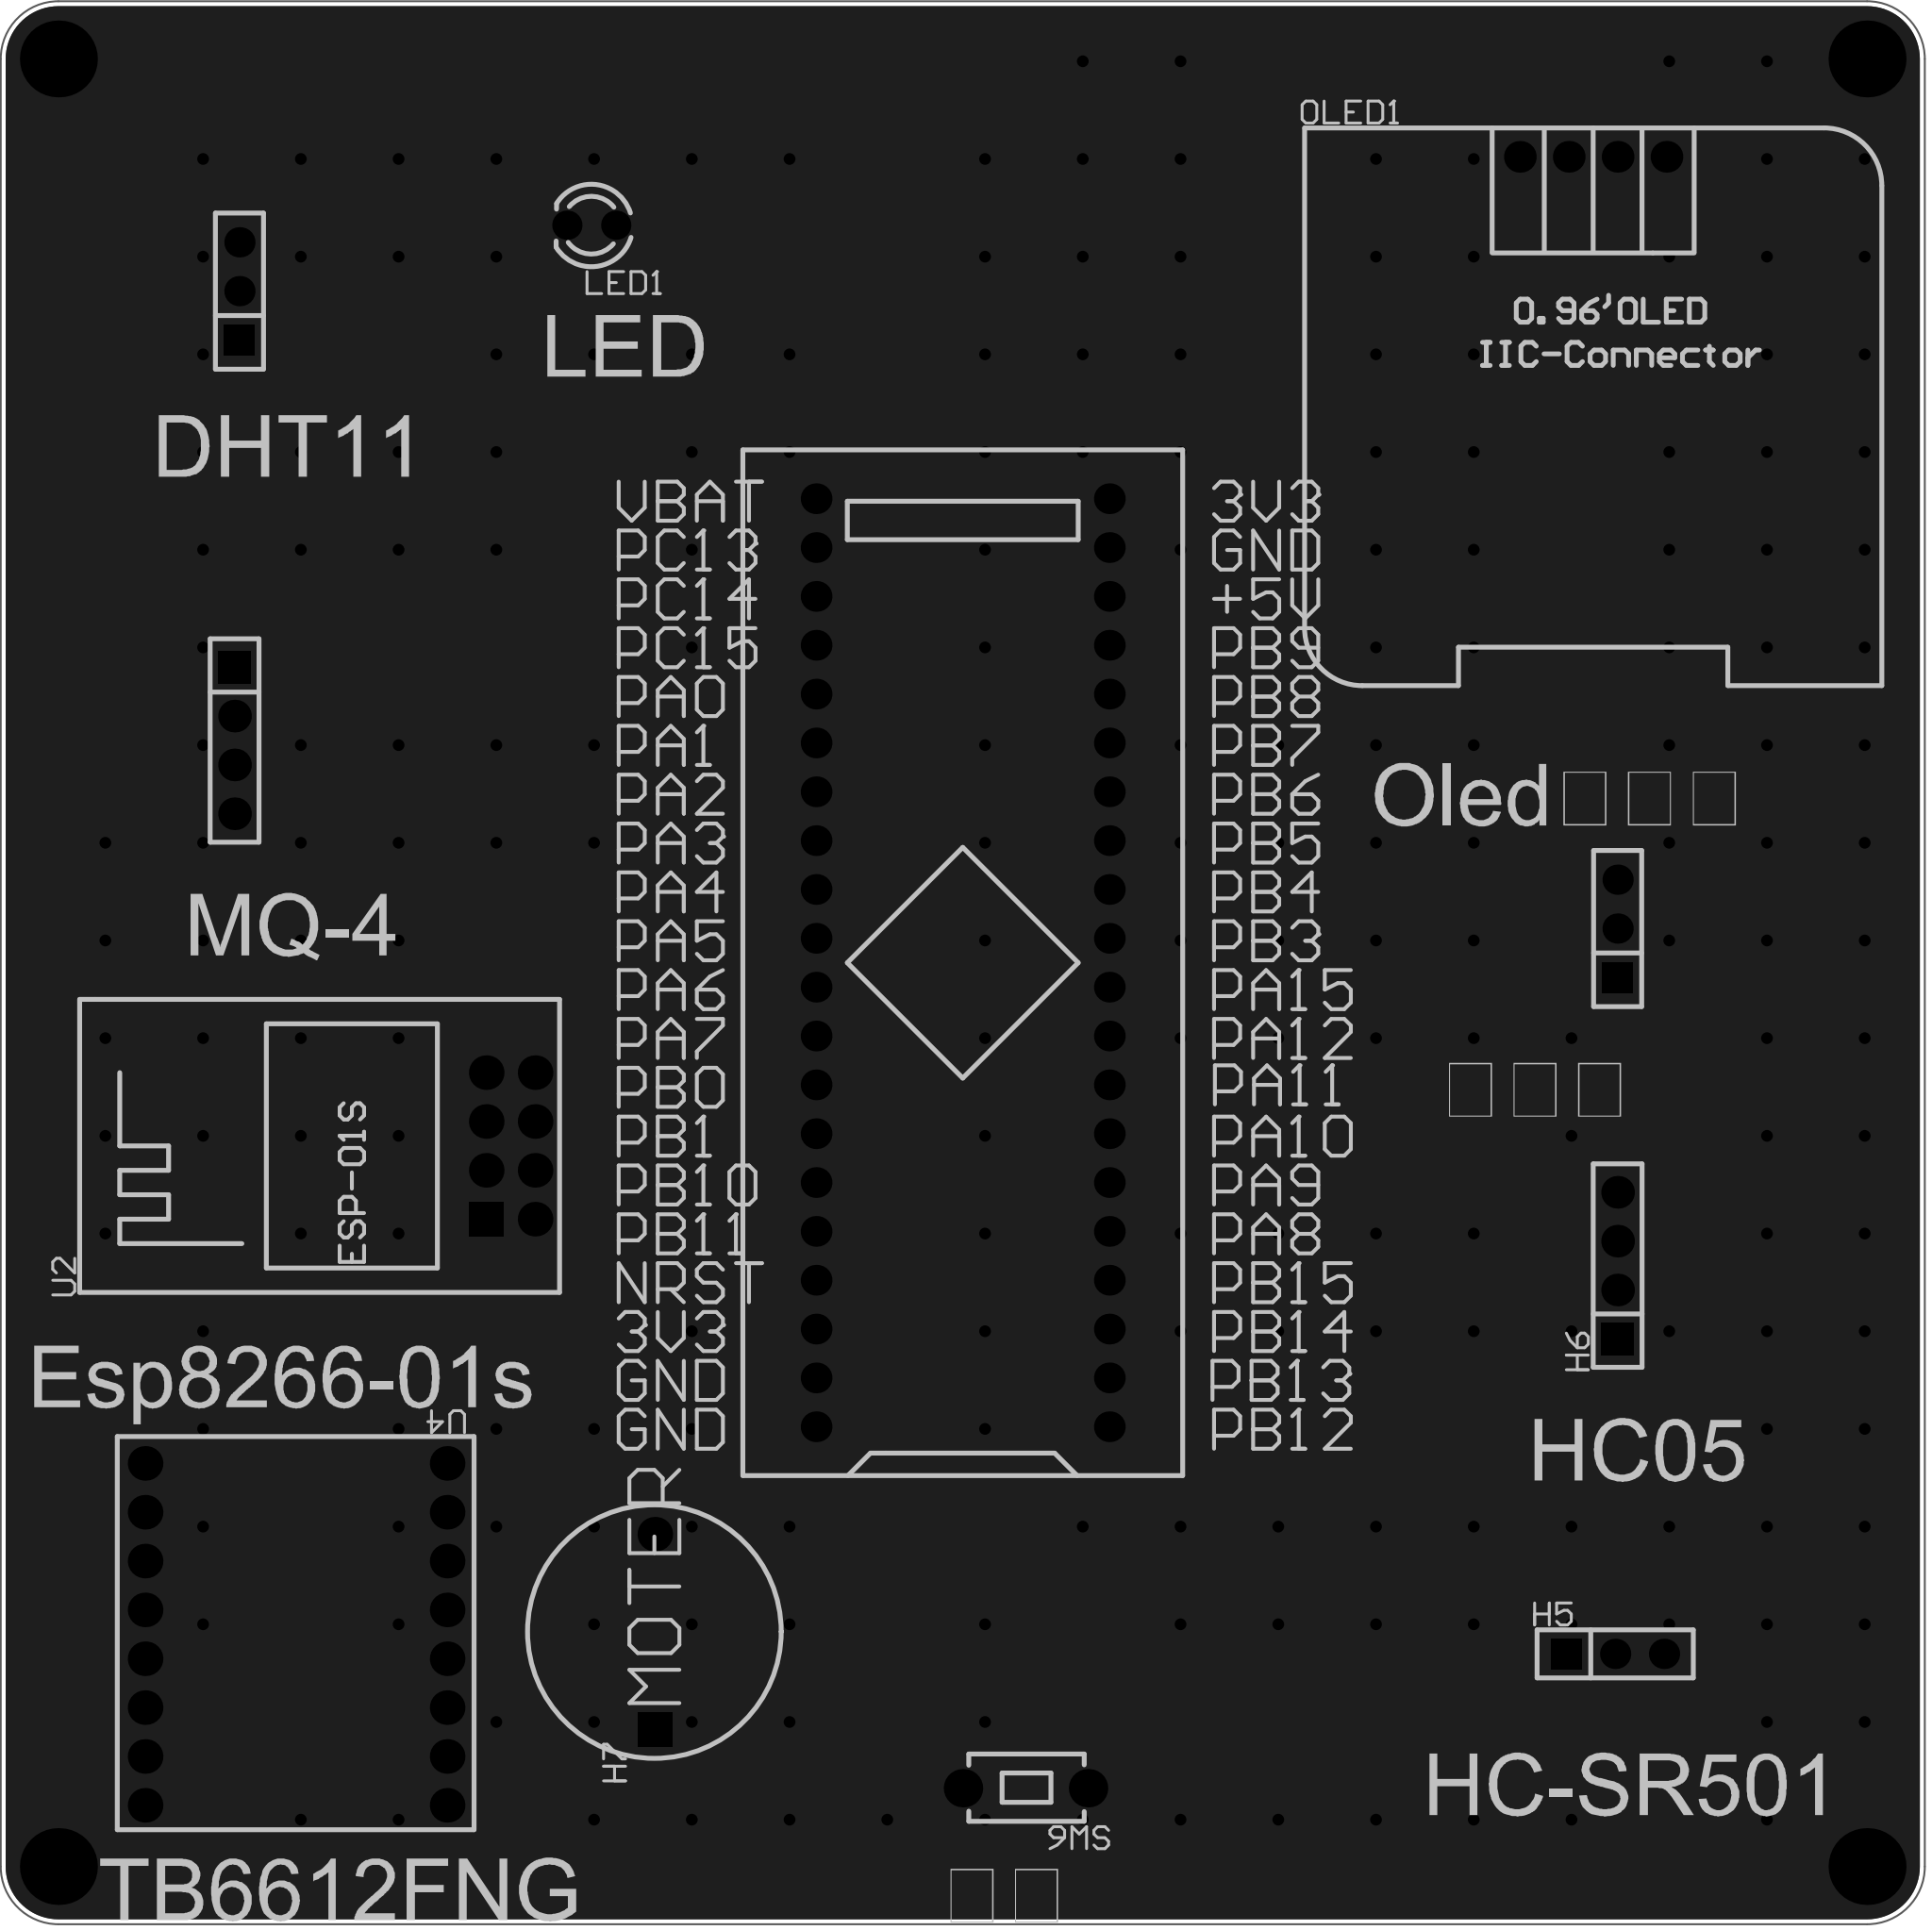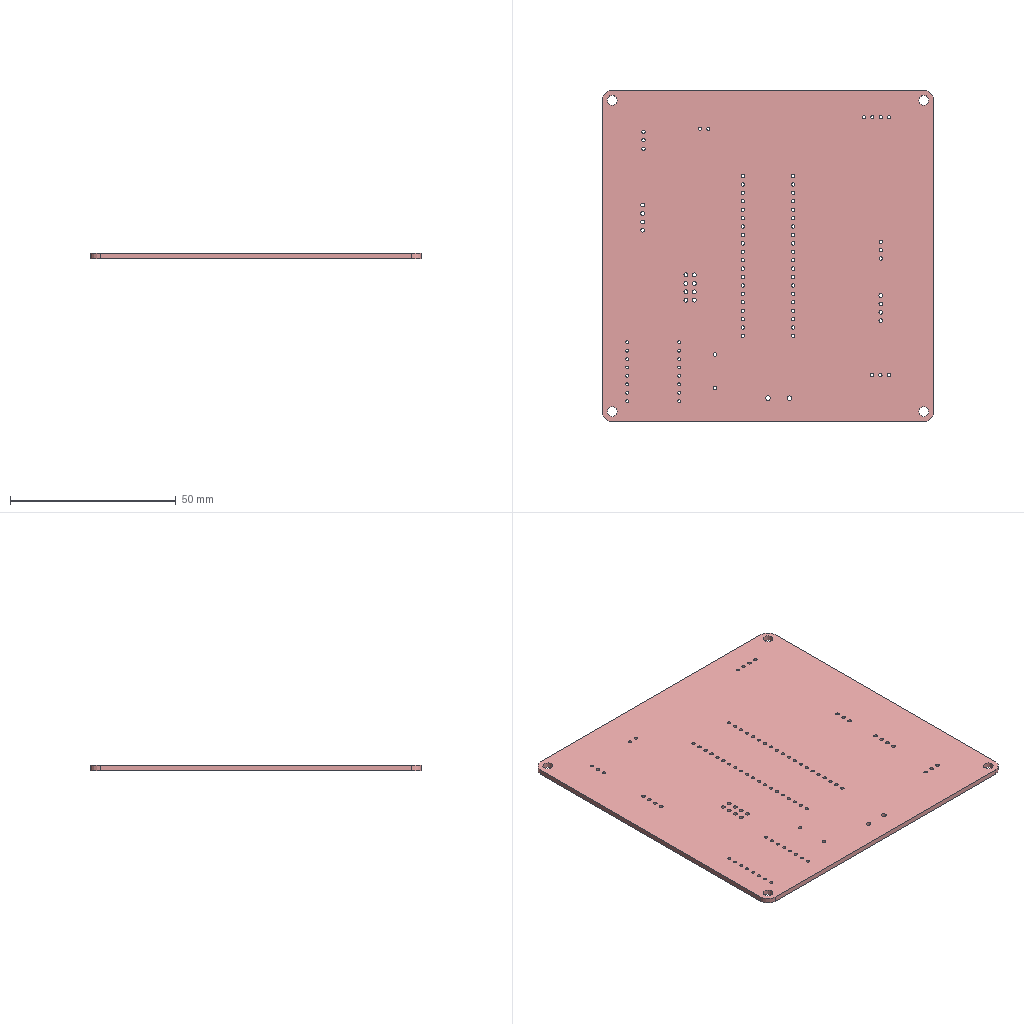Circuit board layout | Altium Designer | box 100 x 100 x 1.6 mm
Layer stack:
# Altium Designer layer stack of  (unit mm; dielectric type: 0 none, 1 core, 2 prepreg, 3 surface material)
index,name,kind,layer,copper_thickness_mm,dielectric_type,dielectric_thickness_mm,dielectric_material,dielectric_constant
0,Top Paste Mask Layer,other,,,,,,
1,Top Silkscreen Layer,other,,,,,,
2,Top Solder Mask Layer,dielectric,,,3,0.01,,3.3
3,Top Layer,copper,Top Layer,0.035,,,,
4,Dielectric1,dielectric,,,3,1.51,FR4,4.5
5,Bottom Layer,copper,Bottom Layer,0.035,,,,
6,Bottom Solder Mask Layer,dielectric,,,3,0.01,,3.3
7,Bottom Silkscreen Layer,other,,,,,,
8,Bottom Paste Mask Layer,other,,,,,,
# drill layer pairs: low layer,high layer
drill_pair,Top Layer,Bottom Layer
Part placement:
Designator,Comment,Layer,Footprint,Center-X(mm),Center-Y(mm),Rotation
U1,STM32F103C8T6-Card,TopLayer,CONN-TH_L53.3-W22.9_STM32F103C8T6-CARD,141.351,130.937,90
H1,,TopLayer,HDR-TH_3P-P2.54-V-F,175.387,132.715,90
H3,,TopLayer,HDR-TH_3P-P2.54-V-F,103.759,165.862,90
H4,,TopLayer,HDR-TH_4P-P2.54-V-F,103.505,142.494,270
H5,,TopLayer,HDR-TH_3P-P2.54-V-F,175.26,94.996,0
H6,,TopLayer,HDR-TH_4P-P2.54-V-F,175.387,115.189,90
LED1,,TopLayer,LED_TH-3mm,122.047,169.291,180
OLED1,,TopLayer,0.96OLED_4P,174.117,172.847,0
U2,ESP-01S,TopLayer,WIFIM-TH_ESP-01S,117.856,121.412,90
U4,,TopLayer,tb6612,106.705,96.012,180
H7,,TopLayer,HDR-TH_2P-P2.54-V-M-1,125.349,96.139,90
SW6,,TopLayer,Key_TH_3.5x6x4.3,144.615,88.011,180
Pad and via stacks:
# Altium Designer via and pad stacks of  (unit mm). Each distinct definition once, with the count of objects using it.
# via: kind,start_layer,end_layer,hole_mm,diameter_mm,mode(0 simple;1 top-mid-bottom;2 full stack),diameter_per_layer,count,example_net
# pad: kind,layer,hole_mm,hole_type(0 round;1 square;2 slot),plating,top_size,top_shape(1 round;2 rect;3 octagon;9 rounded rect),mid_size,bottom_size,mode,footprint,size_per_layer,count,example
pad,Multi-Layer,3,0,plated,4x4,1,4x4,4x4,0,,,4,1
pad,Multi-Layer,1,0,plated,1.6x1.6,1,1.6x1.6,1.6x1.6,0,CONN-TH_L53.3-W22.9_STM32F103C8T6-CARD,,40,U1.1
pad,Multi-Layer,1.02,0,plated,1.575x1.575,1,1.575x1.575,1.575x1.575,0,HDR-TH_3P-P2.54-V-F,,6,H1.3
pad,Multi-Layer,1.02,0,plated,1.575x1.575,2,1.575x1.575,1.575x1.575,0,HDR-TH_3P-P2.54-V-F,,3,H1.1
pad,Multi-Layer,1.1,0,plated,1.7x1.7,2,1.7x1.7,1.7x1.7,0,HDR-TH_4P-P2.54-V-F,,2,H4.1
pad,Multi-Layer,1.1,0,plated,1.7x1.7,1,1.7x1.7,1.7x1.7,0,HDR-TH_4P-P2.54-V-F,,6,H4.2
pad,Multi-Layer,0.9144,0,plated,1.524x1.524,1,1.524x1.524,1.524x1.524,0,LED_TH-3mm,,2,LED1.1
pad,Multi-Layer,1,0,plated,1.65x1.65,1,1.65x1.65,1.65x1.65,0,0.96OLED_4P,,4,OLED1.4
pad,Multi-Layer,1.2,0,plated,1.8x1.8,2,1.8x1.8,1.8x1.8,0,WIFIM-TH_ESP-01S,,1,U2.1
pad,Multi-Layer,1.2,0,plated,1.8x1.8,1,1.8x1.8,1.8x1.8,0,WIFIM-TH_ESP-01S,,7,U2.2
pad,Multi-Layer,0.9,0,plated,1.8x1.8,1,1.8x1.8,1.8x1.8,0,tb6612,,16,U4.1
pad,Multi-Layer,1.1,0,plated,1.8x1.8,1,1.8x1.8,1.8x1.8,0,HDR-TH_2P-P2.54-V-M-1,,1,H7.2
pad,Multi-Layer,1.1,0,plated,1.8x1.8,2,1.8x1.8,1.8x1.8,0,HDR-TH_2P-P2.54-V-M-1,,1,H7.1
pad,Multi-Layer,1.399,0,plated,1.999x1.999,1,1.999x1.999,1.999x1.999,0,Key_TH_3.5x6x4.3,,2,SW6.A
via,Top Layer,Bottom Layer,0.3048,0.61,0,,215,GND
Copper pours:
name,layer,net,type(0 solid;1 hatched;2 none)
Bottom Layer-GND,Bottom Layer,GND,0
Top Layer-GND,Top Layer,GND,0
Design rules, without the lines most boards share:
# Altium Designer design rules of  (exported by Altium Designer, unit mm)
# columns: name | kind | enabled | priority | scope1 | scope2 | descriptor | typed fields (field=value)
Copper_copperRegion_copperThickness1oz | 0 | disabled | 4 | All | All | Clearance Constraint (Gap=5.984mil) (Disabled)(All),(All) | gap=0.152
Copper_copperRegion_copperThickness1oz_1 | 63 | disabled | 4 | All | All | Board Clearance Constraint (Gap=0mil) (Disabled)(All) |
Copper_copperRegion_Copper_copperRegion | 0 | disabled | 5 | All | All | Clearance Constraint (Gap=5.984mil) (Disabled)(All),(All) | gap=0.152
Copper_copperRegion_Copper_copperRegion_1 | 63 | disabled | 5 | All | All | Board Clearance Constraint (Gap=0mil) (Disabled)(All) |
copperThickness1oz | 0 | enabled | 6 | All | All | Clearance Constraint (Gap=5.984mil) (All),(All) | gap=0.152
copperThickness1oz_1 | 63 | enabled | 6 | All | All | Board Clearance Constraint (Gap=0mil) (All) |
copperRegion_copperThickness1oz | 20 | disabled | 1 | All | All | Polygon Connect Rule(Relief Connect )(Conductor Width=10mil) (Relief Angle=90 Angle) (Entries=4) (Air Gap Width=10mil) (Disabled)(All),(All) | connect_style(0=relief,1=direct,2=none)=0 relief_conductor_width=0.254 relief_entries=4
copperRegion_Copper_copperRegion | 20 | disabled | 2 | All | All | Polygon Connect Rule(Relief Connect )(Conductor Width=10mil) (Relief Angle=90 Angle) (Entries=4) (Air Gap Width=10mil) (Disabled)(All),(All) | connect_style(0=relief,1=direct,2=none)=0 relief_conductor_width=0.254 relief_entries=4
copperRegion | 20 | enabled | 3 | All | All | Polygon Connect Rule(Relief Connect )(Conductor Width=10mil) (Relief Angle=90 Angle) (Entries=4) (Air Gap Width=10mil) (All),(All) | connect_style(0=relief,1=direct,2=none)=0 relief_conductor_width=0.254 relief_entries=4